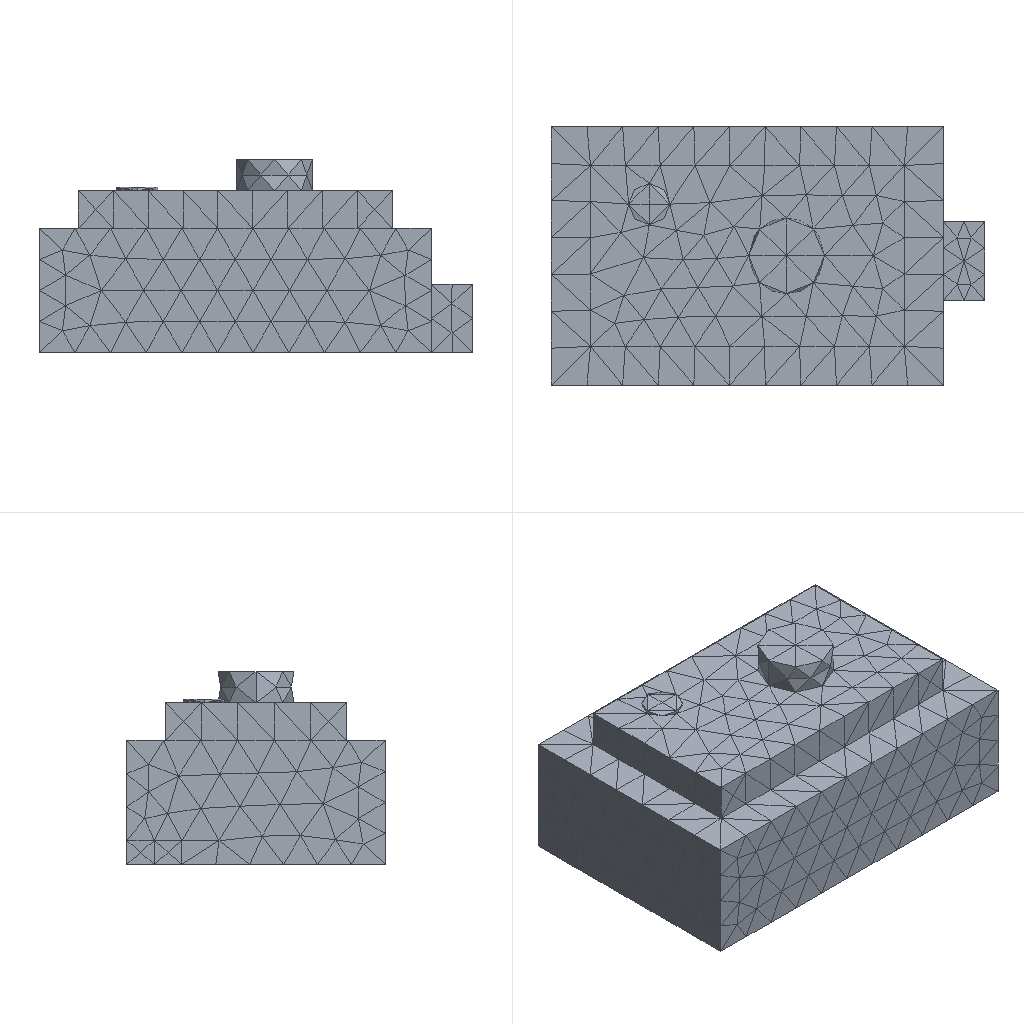Simulation study | ansys mapdl
Set-up summary:
category,name,step,type,value,unit,region
solver,ansys_mapdl
units,mm-N-s-tonne (MPa),,inferred,E=210000 density=
analysis,model,,static
mesh,nodes,,,5331
mesh,elements,,,3258
element_type,SOLID187,,,3258
material,mat 1,,E,210000
material,mat 1,,nu,0.3
load,,model,body load temp,,,all
load,,model,force,"1000 [dir=(0, 0, -1) n=405]",,node list
bc,,model,fixed,"[dofs=UX,UY,UZ n=5774]",,node list
Ansys APDL input file, long lists of numbers shortened:
/COM,ANSYS RELEASE 2026 R1           BUILD 26.1      UP20260202       09:09:58
/PREP7
/NOPR
/TITLE,2
ANTYPE, 0
*IF,_CDRDOFF,EQ,1,THEN     !if solid model was read in
_CDRDOFF=             !reset flag, numoffs already performed
*ELSE              !offset database for the following FE model
NUMOFF,NODE,     5331
NUMOFF,ELEM,     3258
NUMOFF,MAT ,        1
NUMOFF,TYPE,        1
*ENDIF
*SET,_RETURN ,  0.
*SET,_STATUS ,  0.
*SET,_UIQR   ,  405.
*SET,__FLOATPARAMETER__,  5331.
DOF,DELETE
ETBLOCK,        1,        1
(2i9,19a9)
        1      187        0        0        0        0        0        0        0        0        0        0        0        0        0        0        0        0        0        0        0
       -1
NBLOCK,6,SOLID,      5331,      5331
(3i9,6e21.13e3)
        1        0        0-4.0900000000000E+001 3.7500000000000E+001 7.0000000000000E+000
! (5330 more lines like these left out)
N,UNBL,LOC,       -1,
EBLOCK,19,SOLID,      3258,      3258
(19i10)
         1         1         1         1         0         0         0         0        10         0         1      1875      1876      1877      1878      2208      2209      2210      2211
! (6515 more lines like these left out)
        -1
MPTEMP,UNBL, 1, 1,  0.    ,
MPDATA,UNBL, 1,EX  ,       1, 1,  210000.000    ,
MPTEMP,UNBL, 1, 1,  0.    ,
MPDATA,UNBL, 1,NUXY,       1, 1, 0.3    ,
MPTEMP,UNBL, 1, 1,  0.    ,
MPDATA,UNBL, 1,PRXY,       1, 1, 0.3    ,
EXTOPT,ATTR,      0,      0,      0
EXTOPT,ESIZE,  0,  0.
EXTOPT,ACLEAR,      0
TREF,  0.
IRLF,  0
BFUNIF,TEMP,_TINY
ACEL,  0.    ,  0.    ,  0.
OMEGA,  0.    ,  0.    ,  0.
DOMEGA,  0.    ,  0.    ,  0.
CGLOC,  0.    ,  0.    ,  0.
CGOMEGA,  0.    ,  0.    ,  0.
DCGOMG,  0.    ,  0.    ,  0.
KUSE,     0
TIME,  0.
ALPHAD,  0.
BETAD,  0.
DMPRAT,  0.
DMPSTR,  0.
CRPLIM, 0.1    ,   0
CRPLIM,  0.    ,   1
NCNV,     0, 1.000000000E+12,     0,  0.    ,  0.
NEQIT,     0
ERESX,DEFA
DBLOCK,      5774
(i9,a6,2(pg16.9))
        1  UX    0.00000000      0.00000000
! (5773 more lines like these left out)
       -1
FBLOCK,       405
(i9,a6,2(pg16.9))
      588  FZ   -2.46913580      0.00000000
! (404 more lines like these left out)
       -1
/GO
FINISH
Results summary:
result,analysis_type_db,,,static,unstated
result,n_sets,,,1,unstated
result,load_steps[0].set,load_step=1,,1,unstated
result,load_steps[0].substep,load_step=1,,1,unstated
result,load_steps[0].time,load_step=1,,1,unstated
result,load_steps[0].freq,load_step=1,,1,unstated
result,load_steps[0].max_usum,load_step=1,,0.0001339,unstated
result,load_steps[0].max_seqv,load_step=1,,10.543,unstated
result,load_steps[0].reaction_sum.FX,load_step=1,,-3.70903e-12,unstated
result,load_steps[0].reaction_sum.FY,load_step=1,,-1.35536e-11,unstated
result,load_steps[0].reaction_sum.FZ,load_step=1,,1000,unstated
result,load_steps[0].reaction_sum.MX,load_step=1,,0,unstated
result,load_steps[0].reaction_sum.MY,load_step=1,,0,unstated
result,load_steps[0].reaction_sum.MZ,load_step=1,,0,unstated
result,convergence,,,results present for all listed sets,unstated